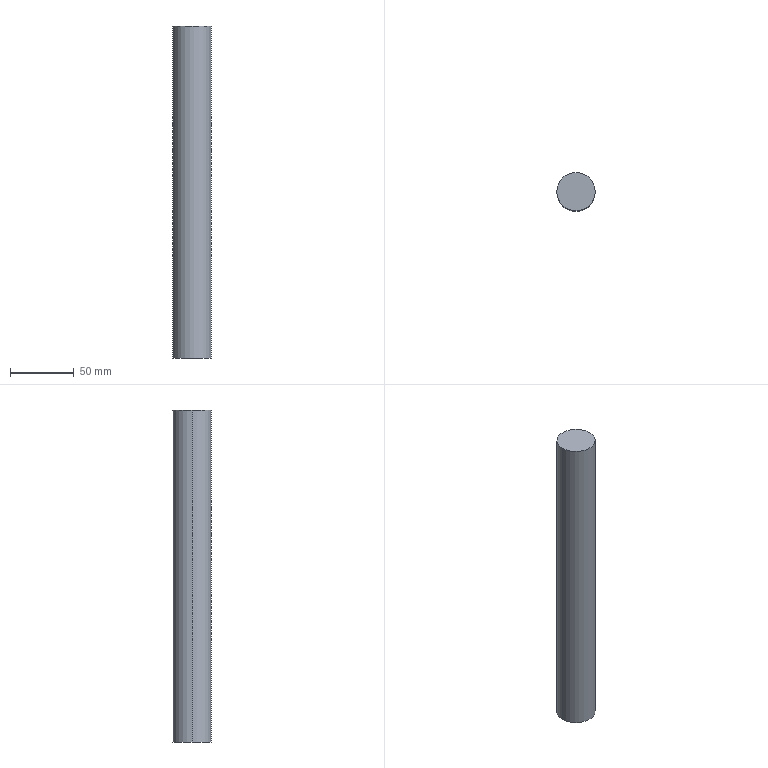Part | STEP file | MYT-A01-P33 | 1 solid | 4 faces | box 30 x 30 x 260 mm | volume 183783 mm3 | cylinder 2 | plane 2 | commonest cylinder face diameters 30 x2
STEP:
#1=CARTESIAN_POINT('',(15.,0.,260.));
#2=VERTEX_POINT('',#1);
#3=CARTESIAN_POINT('',(-15.,0.,260.));
#4=VERTEX_POINT('',#3);
#5=CARTESIAN_POINT('',(0.,0.,260.));
#6=DIRECTION('',(0.,0.,1.));
#7=DIRECTION('',(1.,0.,0.));
#8=AXIS2_PLACEMENT_3D('',#5,#6,#7);
#9=CIRCLE('',#8,15.);
#10=EDGE_CURVE('',#2,#4,#9,.T.);
#11=ORIENTED_EDGE('',*,*,#10,.F.);
#12=CARTESIAN_POINT('',(15.,0.,0.));
#13=VERTEX_POINT('',#12);
#14=CARTESIAN_POINT('',(15.,0.,260.));
#15=DIRECTION('',(0.,0.,-1.));
#16=VECTOR('',#15,1000.);
#17=LINE('',#14,#16);
#18=EDGE_CURVE('',#2,#13,#17,.T.);
#19=ORIENTED_EDGE('',*,*,#18,.T.);
#20=CARTESIAN_POINT('',(-15.,0.,0.));
#21=VERTEX_POINT('',#20);
#22=CARTESIAN_POINT('',(0.,0.,0.));
#23=DIRECTION('',(0.,0.,1.));
#24=DIRECTION('',(1.,0.,0.));
#25=AXIS2_PLACEMENT_3D('',#22,#23,#24);
#26=CIRCLE('',#25,15.);
#27=EDGE_CURVE('',#13,#21,#26,.T.);
#28=ORIENTED_EDGE('',*,*,#27,.T.);
#29=CARTESIAN_POINT('',(-15.,0.,260.));
#30=DIRECTION('',(0.,0.,-1.));
#31=VECTOR('',#30,1000.);
#32=LINE('',#29,#31);
#33=EDGE_CURVE('',#4,#21,#32,.T.);
#34=ORIENTED_EDGE('',*,*,#33,.F.);
#35=EDGE_LOOP('',(#11,#19,#28,#34));
#36=FACE_OUTER_BOUND('',#35,.T.);
#37=CARTESIAN_POINT('',(0.,0.,260.));
#38=DIRECTION('',(0.,0.,-1.));
#39=DIRECTION('',(-1.,0.,0.));
#40=AXIS2_PLACEMENT_3D('',#37,#38,#39);
#41=CYLINDRICAL_SURFACE('',#40,15.);
#42=ADVANCED_FACE('',(#36),#41,.T.);
#43=ORIENTED_EDGE('',*,*,#18,.F.);
#44=CARTESIAN_POINT('',(0.,0.,260.));
#45=DIRECTION('',(0.,0.,1.));
#46=DIRECTION('',(1.,0.,0.));
#47=AXIS2_PLACEMENT_3D('',#44,#45,#46);
#48=CIRCLE('',#47,15.);
#49=EDGE_CURVE('',#4,#2,#48,.T.);
#50=ORIENTED_EDGE('',*,*,#49,.F.);
#51=ORIENTED_EDGE('',*,*,#33,.T.);
#52=CARTESIAN_POINT('',(0.,0.,0.));
#53=DIRECTION('',(0.,0.,1.));
#54=DIRECTION('',(1.,0.,0.));
#55=AXIS2_PLACEMENT_3D('',#52,#53,#54);
#56=CIRCLE('',#55,15.);
#57=EDGE_CURVE('',#21,#13,#56,.T.);
#58=ORIENTED_EDGE('',*,*,#57,.T.);
#59=EDGE_LOOP('',(#43,#50,#51,#58));
#60=FACE_OUTER_BOUND('',#59,.T.);
#61=CARTESIAN_POINT('',(0.,0.,260.));
#62=DIRECTION('',(0.,0.,-1.));
#63=DIRECTION('',(-1.,0.,0.));
#64=AXIS2_PLACEMENT_3D('',#61,#62,#63);
#65=CYLINDRICAL_SURFACE('',#64,15.);
#66=ADVANCED_FACE('',(#60),#65,.T.);
#67=ORIENTED_EDGE('',*,*,#49,.T.);
#68=ORIENTED_EDGE('',*,*,#10,.T.);
#69=EDGE_LOOP('',(#67,#68));
#70=FACE_OUTER_BOUND('',#69,.T.);
#71=CARTESIAN_POINT('',(0.,0.,260.));
#72=DIRECTION('',(0.,0.,1.));
#73=DIRECTION('',(1.,0.,0.));
#74=AXIS2_PLACEMENT_3D('',#71,#72,#73);
#75=PLANE('',#74);
#76=ADVANCED_FACE('',(#70),#75,.T.);
#77=ORIENTED_EDGE('',*,*,#57,.F.);
#78=ORIENTED_EDGE('',*,*,#27,.F.);
#79=EDGE_LOOP('',(#77,#78));
#80=FACE_OUTER_BOUND('',#79,.T.);
#81=CARTESIAN_POINT('',(0.,0.,0.));
#82=DIRECTION('',(0.,0.,1.));
#83=DIRECTION('',(1.,0.,0.));
#84=AXIS2_PLACEMENT_3D('',#81,#82,#83);
#85=PLANE('',#84);
#86=ADVANCED_FACE('',(#80),#85,.F.);
#87=CLOSED_SHELL('',(#42,#66,#76,#86));
#88=MANIFOLD_SOLID_BREP('',#87);
#89=CARTESIAN_POINT('',(0.,0.,0.));
#90=DIRECTION('',(0.,0.,1.));
#91=DIRECTION('',(1.,0.,0.));
#92=AXIS2_PLACEMENT_3D('',#89,#90,#91);
#93=(LENGTH_UNIT()NAMED_UNIT(*)SI_UNIT(.MILLI.,.METRE.));
#94=UNCERTAINTY_MEASURE_WITH_UNIT(LENGTH_MEASURE(0.00001),#93,'','');
#95=(NAMED_UNIT(*)PLANE_ANGLE_UNIT()SI_UNIT($,.RADIAN.));
#96=(NAMED_UNIT(*)SI_UNIT($,.STERADIAN.)SOLID_ANGLE_UNIT());
#97=(GEOMETRIC_REPRESENTATION_CONTEXT(3)GLOBAL_UNCERTAINTY_ASSIGNED_CONTEXT((#94))GLOBAL_UNIT_ASSIGNED_CONTEXT((#93,#95,#96))REPRESENTATION_CONTEXT('',''));
#98=ADVANCED_BREP_SHAPE_REPRESENTATION('',(#88,#92),#97);